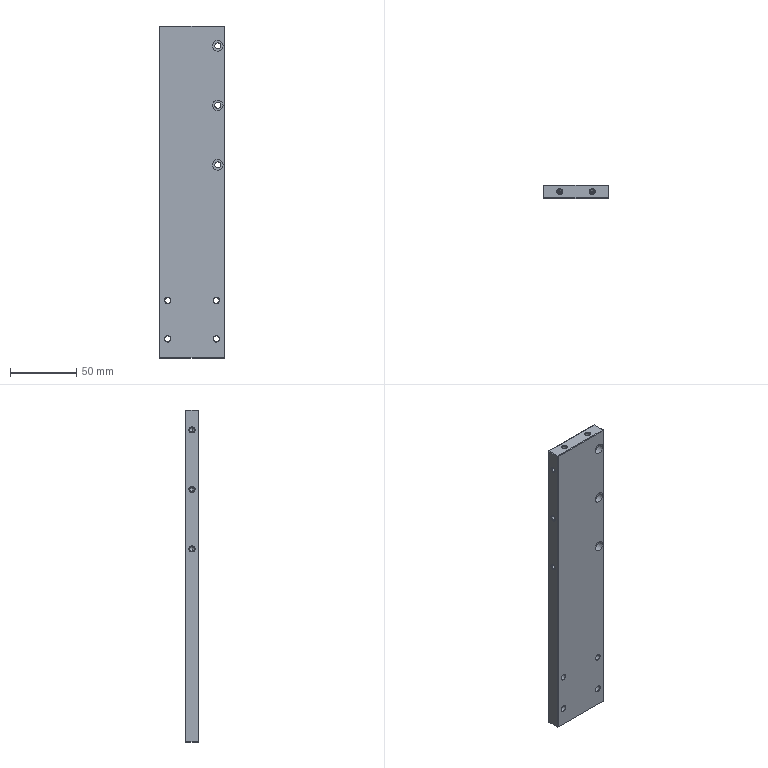Part | NX | 1 solid | 89 faces | box 49 x 10 x 251 mm | volume 120813 mm3 | cylinder 40 | cone 28 | plane 21 | commonest cylinder face diameters 3.3 x20 4.5 x14 8 x6